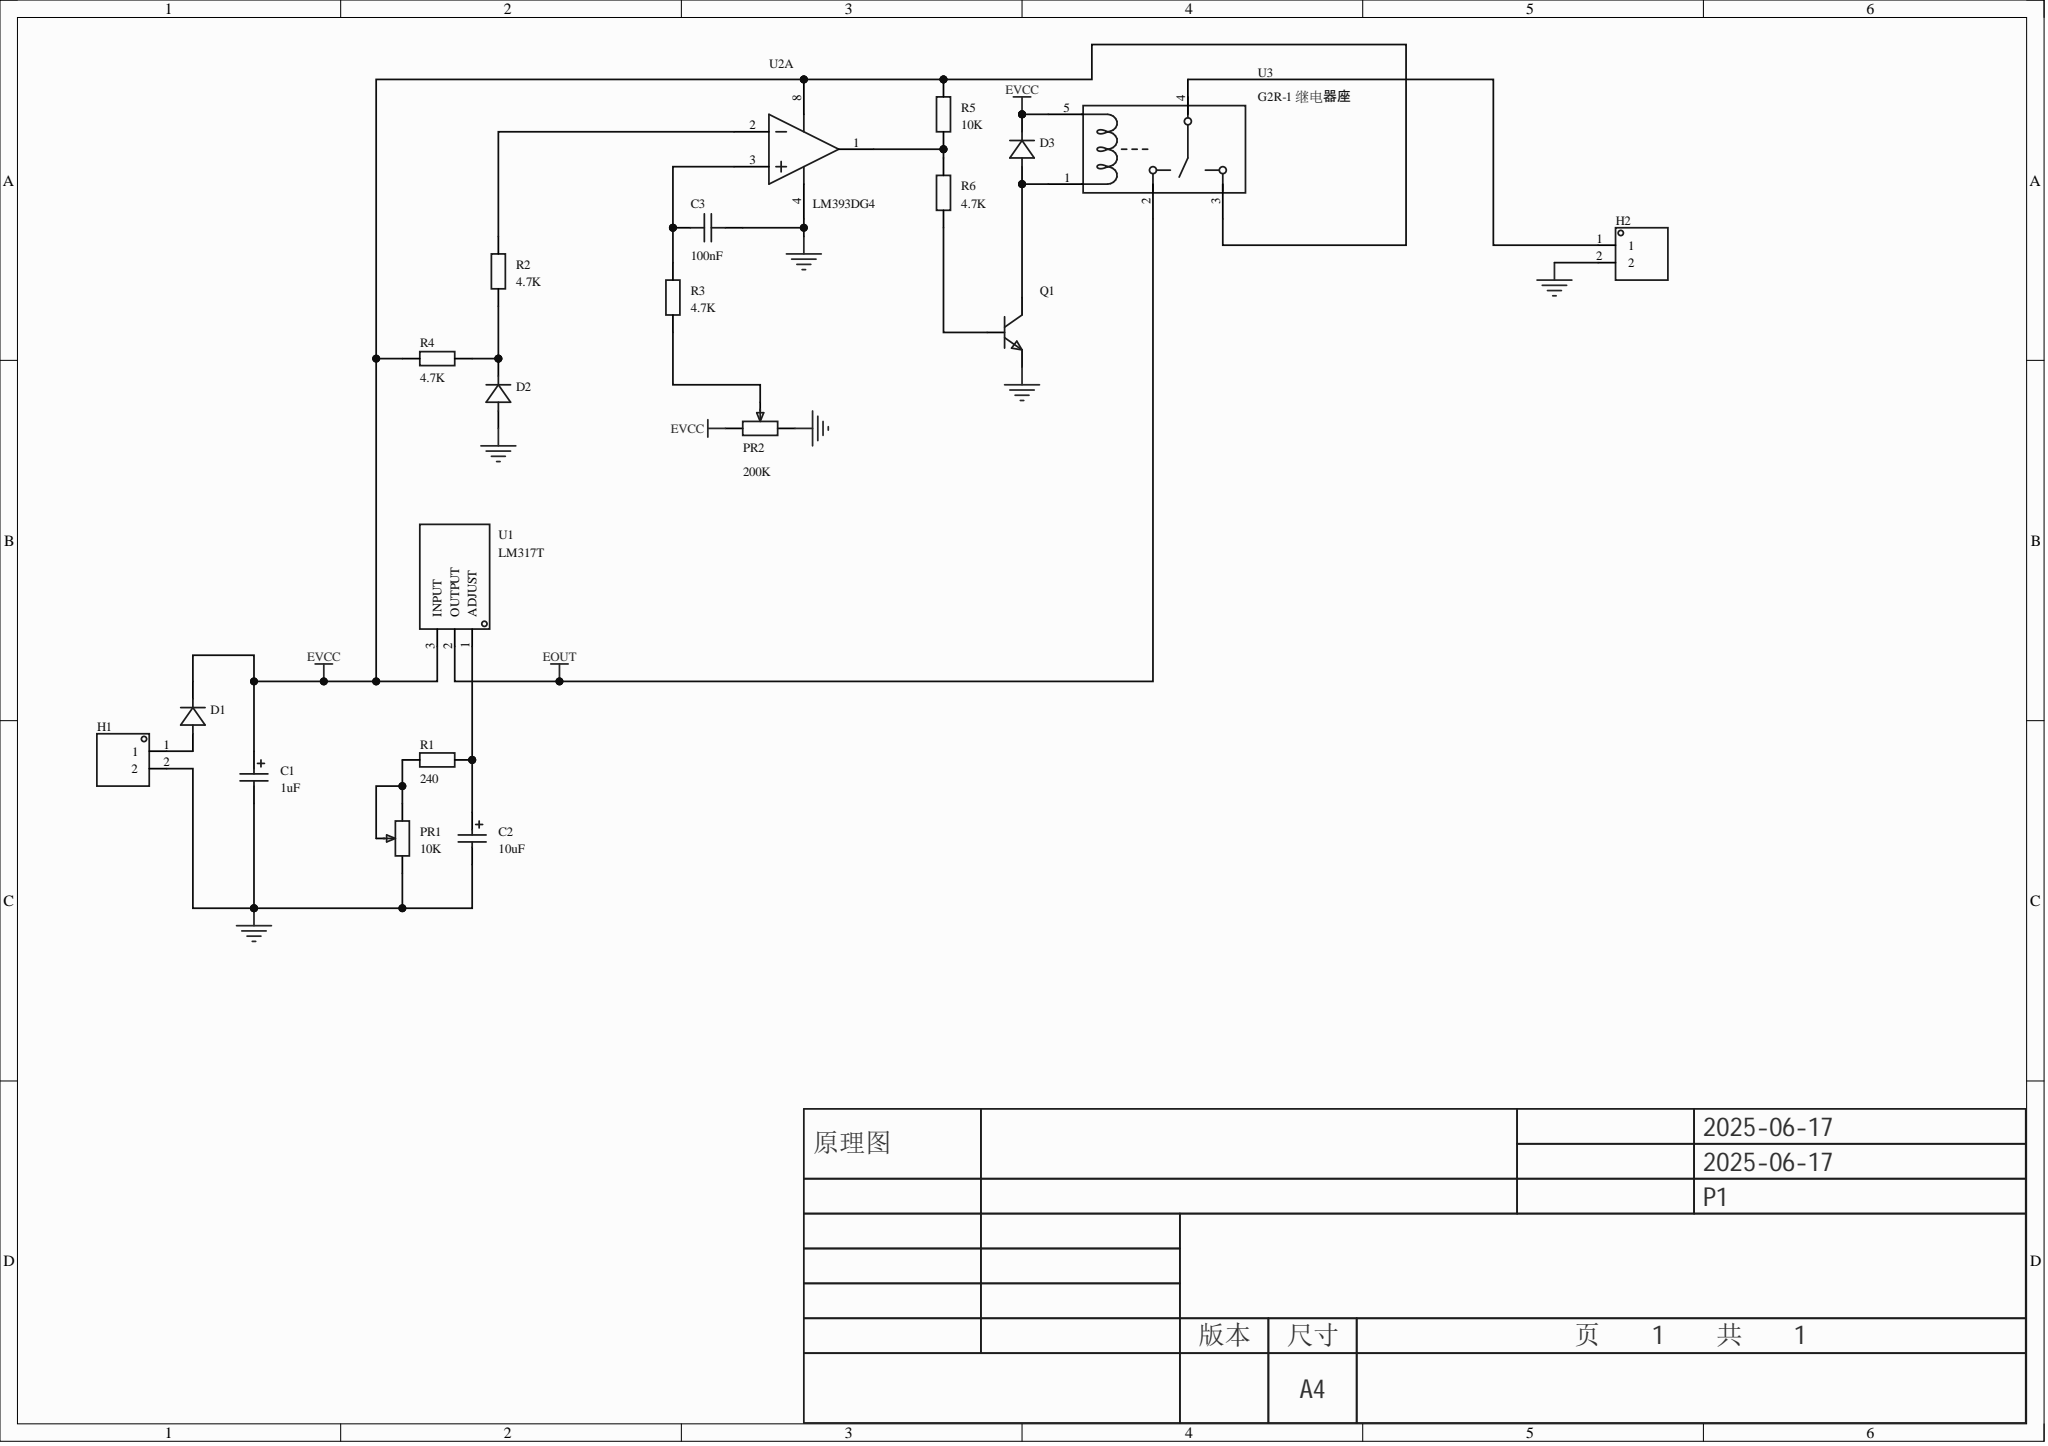Circuit board | Altium Designer | 20 parts | 14 nets
Bill of materials:
Comment,Description,Designator,Footprint,LibRef,Quantity
"1uF","","C1","C_Ele_SMD_3x5.4mm","C_Ele_SMD_3x5.4mm","1"
"10uF","","C2","C_Ele_SMD_3x5.4mm","C_Ele_SMD_3x5.4mm","1"
"100nF","","C3","C0603","CAP_0603","1"
"","","D1, D2, D3","DO_1N4007","D_1N4007A","3"
"","","H1, H2","HDR-TH_2P-P2.54-V-M-1","HDR-M_2.54_1x2P","2"
"10K","","PR1","R_3386P","R_3386P","1"
"200K","","PR2","R_3386P","R_3386P","1"
"","","Q1","S8050_SOT-23","S8050_SOT_NPN","1"
"240","","R1","R0603","Res_0603","1"
"4.7K","","R2, R3, R4, R6","R0603","Res_0603","4"
"10K","","R5","R0603","Res_0603","1"
"LM317T","","U1","TO-220-3_L10.2-W4.6-P2.54-L","LM317T","1"
"LM393DG4","","U2","SOIC-8_L4.9-W3.9-P1.27-LS6.0-BL","LM393DG4","1"
"G2R-1 继电器座","","U3","RELAY-TH_G2R-1_C9900014679","G2R-1 继电器座","1"
Netlist (Protel format):
[
C1
C_Ele_SMD_3x5.4mm
1uF



]
[
C2
C_Ele_SMD_3x5.4mm
10uF



]
[
C3
C0603
100nF



]
[
D1
DO_1N4007




]
[
D2
DO_1N4007




]
[
D3
DO_1N4007




]
[
H1
HDR-TH_2P-P2.54-V-M-1




]
[
H2
HDR-TH_2P-P2.54-V-M-1




]
[
PR1
R_3386P
10K



]
[
PR2
R_3386P
200K



]
[
Q1
S8050_SOT-23




]
[
R1
R0603
240



]
[
R2
R0603
4.7K



]
[
R3
R0603
4.7K



]
[
R4
R0603
4.7K



]
[
R5
R0603
10K



]
[
R6
R0603
4.7K



]
[
U1
TO-220-3_L10.2-W4.6-P2.54-L
LM317T



]
[
U2
SOIC-8_L4.9-W3.9-P1.27-LS6.0-BL
LM393DG4



]
[
U3
RELAY-TH_G2R-1_C9900014679
G2R-1 继电器座



]
(
NetR5_1
R5-1
R6-2
U2-1
)
(
NetR2_2
R2-2
U2-2
)
(
NetQ1_1
Q1-1
R6-1
)
(
NetPR2_2
PR2-2
R3-1
)
(
NetPR1_1
PR1-1
PR1-2
R1-1
)
(
NetH2_1
H2-1
U3-4
)
(
NetD3_2
D3-2
Q1-3
U3-1
)
(
NetD2_1
D2-1
R2-1
R4-1
)
(
NetD1_2
D1-2
H1-1
)
(
NetC3_1
C3-1
R3-2
U2-3
)
(
NetC2_1
C2-1
R1-2
U1-1
)
(
GND
C1-2
C2-2
C3-2
D2-2
H1-2
H2-2
PR1-3
PR2-1
Q1-2
U2-4
)
(
EVCC
C1-1
D1-1
D3-1
PR2-3
R4-2
R5-2
U1-3
U2-8
U3-3
U3-5
)
(
EOUT
U1-2
U3-2
)